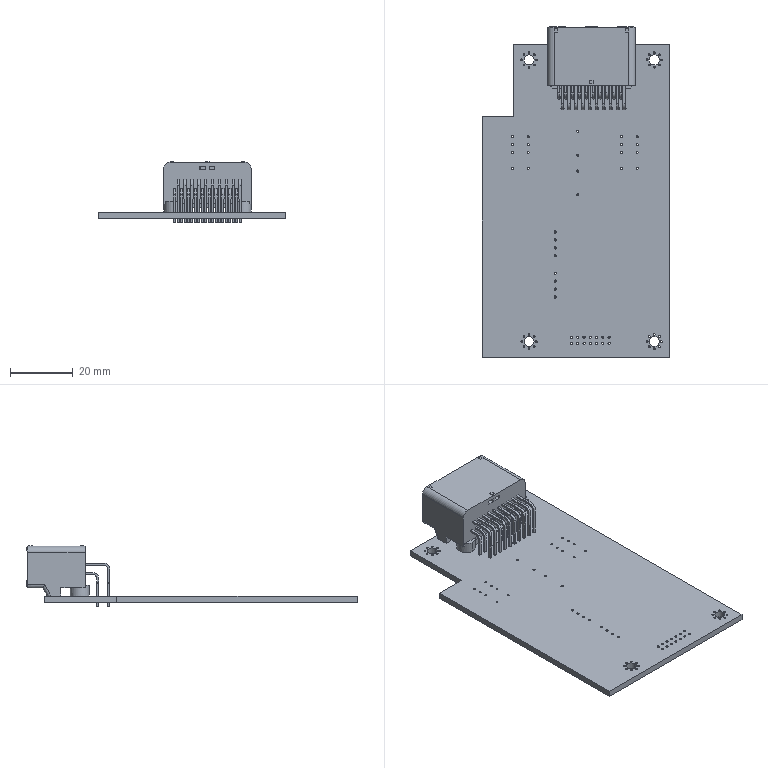Part | SolidWorks | 2 solids | 720 faces | box 60 x 105.587 x 19.2 mm | volume 14940 mm3 | plane 460 | cylinder 260 | commonest cylinder face diameters 0.6 x96 0.7 x52 1 x44 2.64 x20 3.92 x20 3.2 x12